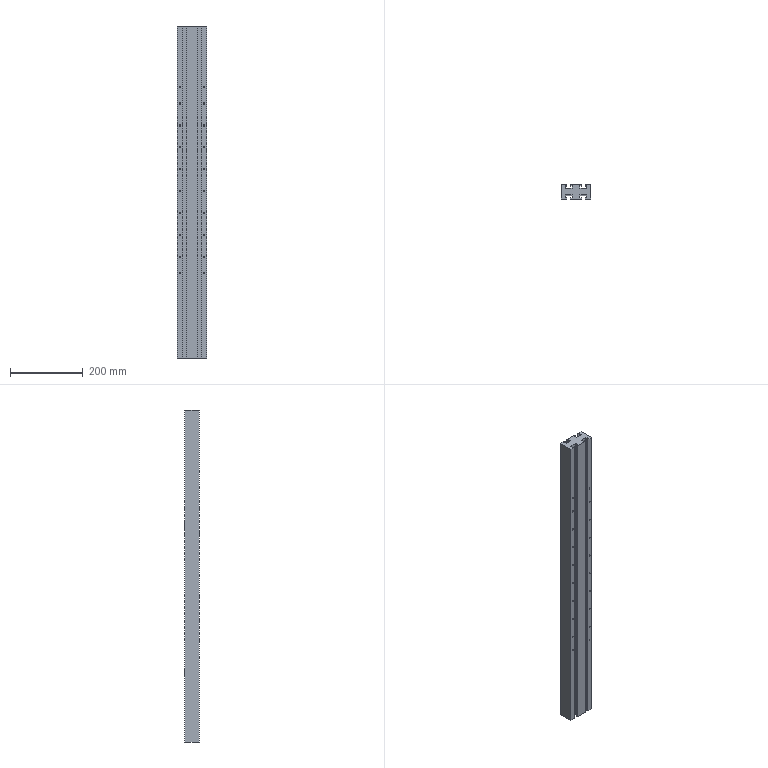Part | 1 solid | 172 faces | box 80 x 40 x 910 mm | volume 2252972 mm3 | cylinder 76 | plane 56 | cone 40 | commonest cylinder face diameters 3.3 x40 3.641 x32 16 x4